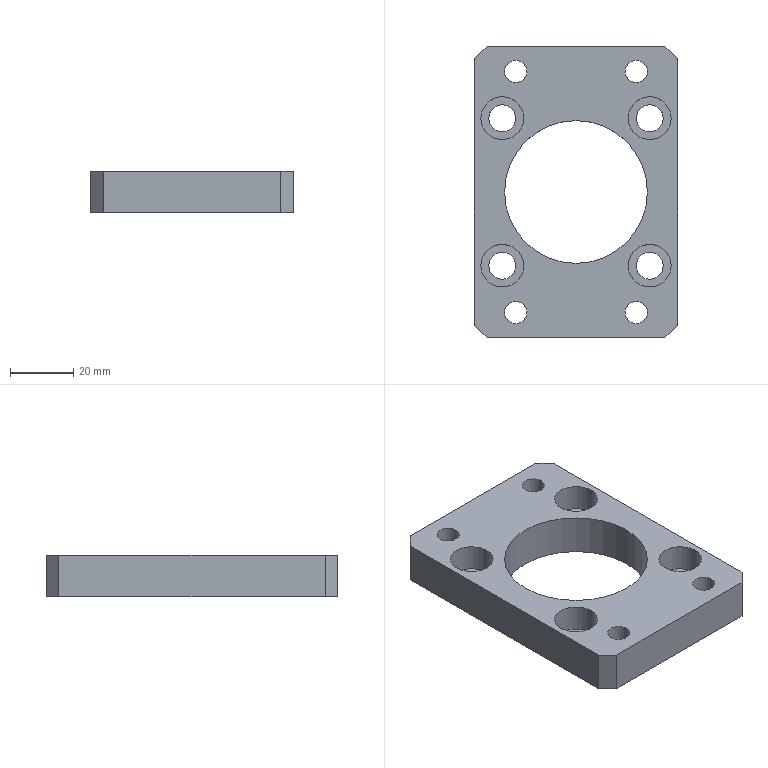Part | SolidWorks | features BaseBody 1 | 1 solid | 40 faces | box 64 x 92 x 13 mm | volume 47563 mm3 | cylinder 26 | plane 14 | commonest cylinder face diameters 7 x8 8.5 x8 13.5 x8 45 x2
STEP:
#1=CARTESIAN_POINT('',(22.5,0.,0.));
#2=VERTEX_POINT('',#1);
#3=CARTESIAN_POINT('',(-22.5,0.,0.));
#4=VERTEX_POINT('',#3);
#5=CARTESIAN_POINT('',(0.,0.,0.));
#6=DIRECTION('',(0.,0.,-1.));
#7=DIRECTION('',(1.,0.,0.));
#8=AXIS2_PLACEMENT_3D('',#5,#6,#7);
#9=CIRCLE('',#8,22.5);
#10=EDGE_CURVE('',#2,#4,#9,.T.);
#11=ORIENTED_EDGE('',*,*,#10,.T.);
#12=CARTESIAN_POINT('',(-22.5,0.,13.));
#13=VERTEX_POINT('',#12);
#14=CARTESIAN_POINT('',(-22.5,0.,0.));
#15=DIRECTION('',(0.,0.,1.));
#16=VECTOR('',#15,1000.);
#17=LINE('',#14,#16);
#18=EDGE_CURVE('',#4,#13,#17,.T.);
#19=ORIENTED_EDGE('',*,*,#18,.T.);
#20=CARTESIAN_POINT('',(22.5,0.,13.));
#21=VERTEX_POINT('',#20);
#22=CARTESIAN_POINT('',(0.,0.,13.));
#23=DIRECTION('',(0.,0.,-1.));
#24=DIRECTION('',(1.,0.,0.));
#25=AXIS2_PLACEMENT_3D('',#22,#23,#24);
#26=CIRCLE('',#25,22.5);
#27=EDGE_CURVE('',#21,#13,#26,.T.);
#28=ORIENTED_EDGE('',*,*,#27,.F.);
#29=CARTESIAN_POINT('',(22.5,0.,0.));
#30=DIRECTION('',(0.,0.,1.));
#31=VECTOR('',#30,1000.);
#32=LINE('',#29,#31);
#33=EDGE_CURVE('',#2,#21,#32,.T.);
#34=ORIENTED_EDGE('',*,*,#33,.F.);
#35=EDGE_LOOP('',(#11,#19,#28,#34));
#36=FACE_OUTER_BOUND('',#35,.T.);
#37=CARTESIAN_POINT('',(0.,0.,0.));
#38=DIRECTION('',(0.,0.,1.));
#39=DIRECTION('',(1.,0.,0.));
#40=AXIS2_PLACEMENT_3D('',#37,#38,#39);
#41=CYLINDRICAL_SURFACE('',#40,22.5);
#42=ADVANCED_FACE('',(#36),#41,.F.);
#43=CARTESIAN_POINT('',(-15.5,38.,0.));
#44=VERTEX_POINT('',#43);
#45=CARTESIAN_POINT('',(-22.5,38.,0.));
#46=VERTEX_POINT('',#45);
#47=CARTESIAN_POINT('',(-19.,38.,0.));
#48=DIRECTION('',(0.,0.,-1.));
#49=DIRECTION('',(1.,0.,0.));
#50=AXIS2_PLACEMENT_3D('',#47,#48,#49);
#51=CIRCLE('',#50,3.5);
#52=EDGE_CURVE('',#44,#46,#51,.T.);
#53=ORIENTED_EDGE('',*,*,#52,.T.);
#54=CARTESIAN_POINT('',(-22.5,38.,13.));
#55=VERTEX_POINT('',#54);
#56=CARTESIAN_POINT('',(-22.5,38.,0.));
#57=DIRECTION('',(0.,0.,1.));
#58=VECTOR('',#57,1000.);
#59=LINE('',#56,#58);
#60=EDGE_CURVE('',#46,#55,#59,.T.);
#61=ORIENTED_EDGE('',*,*,#60,.T.);
#62=CARTESIAN_POINT('',(-15.5,38.,13.));
#63=VERTEX_POINT('',#62);
#64=CARTESIAN_POINT('',(-19.,38.,13.));
#65=DIRECTION('',(0.,0.,-1.));
#66=DIRECTION('',(1.,0.,0.));
#67=AXIS2_PLACEMENT_3D('',#64,#65,#66);
#68=CIRCLE('',#67,3.5);
#69=EDGE_CURVE('',#63,#55,#68,.T.);
#70=ORIENTED_EDGE('',*,*,#69,.F.);
#71=CARTESIAN_POINT('',(-15.5,38.,0.));
#72=DIRECTION('',(0.,0.,1.));
#73=VECTOR('',#72,1000.);
#74=LINE('',#71,#73);
#75=EDGE_CURVE('',#44,#63,#74,.T.);
#76=ORIENTED_EDGE('',*,*,#75,.F.);
#77=EDGE_LOOP('',(#53,#61,#70,#76));
#78=FACE_OUTER_BOUND('',#77,.T.);
#79=CARTESIAN_POINT('',(-19.,38.,0.));
#80=DIRECTION('',(0.,0.,1.));
#81=DIRECTION('',(1.,0.,0.));
#82=AXIS2_PLACEMENT_3D('',#79,#80,#81);
#83=CYLINDRICAL_SURFACE('',#82,3.5);
#84=ADVANCED_FACE('',(#78),#83,.F.);
#85=CARTESIAN_POINT('',(-15.5,-38.,0.));
#86=VERTEX_POINT('',#85);
#87=CARTESIAN_POINT('',(-22.5,-38.,0.));
#88=VERTEX_POINT('',#87);
#89=CARTESIAN_POINT('',(-19.,-38.,0.));
#90=DIRECTION('',(0.,0.,-1.));
#91=DIRECTION('',(1.,0.,0.));
#92=AXIS2_PLACEMENT_3D('',#89,#90,#91);
#93=CIRCLE('',#92,3.5);
#94=EDGE_CURVE('',#86,#88,#93,.T.);
#95=ORIENTED_EDGE('',*,*,#94,.T.);
#96=CARTESIAN_POINT('',(-22.5,-38.,13.));
#97=VERTEX_POINT('',#96);
#98=CARTESIAN_POINT('',(-22.5,-38.,0.));
#99=DIRECTION('',(0.,0.,1.));
#100=VECTOR('',#99,1000.);
#101=LINE('',#98,#100);
#102=EDGE_CURVE('',#88,#97,#101,.T.);
#103=ORIENTED_EDGE('',*,*,#102,.T.);
#104=CARTESIAN_POINT('',(-15.5,-38.,13.));
#105=VERTEX_POINT('',#104);
#106=CARTESIAN_POINT('',(-19.,-38.,13.));
#107=DIRECTION('',(0.,0.,-1.));
#108=DIRECTION('',(1.,0.,0.));
#109=AXIS2_PLACEMENT_3D('',#106,#107,#108);
#110=CIRCLE('',#109,3.5);
#111=EDGE_CURVE('',#105,#97,#110,.T.);
#112=ORIENTED_EDGE('',*,*,#111,.F.);
#113=CARTESIAN_POINT('',(-15.5,-38.,0.));
#114=DIRECTION('',(0.,0.,1.));
#115=VECTOR('',#114,1000.);
#116=LINE('',#113,#115);
#117=EDGE_CURVE('',#86,#105,#116,.T.);
#118=ORIENTED_EDGE('',*,*,#117,.F.);
#119=EDGE_LOOP('',(#95,#103,#112,#118));
#120=FACE_OUTER_BOUND('',#119,.T.);
#121=CARTESIAN_POINT('',(-19.,-38.,0.));
#122=DIRECTION('',(0.,0.,1.));
#123=DIRECTION('',(1.,0.,0.));
#124=AXIS2_PLACEMENT_3D('',#121,#122,#123);
#125=CYLINDRICAL_SURFACE('',#124,3.5);
#126=ADVANCED_FACE('',(#120),#125,.F.);
#127=CARTESIAN_POINT('',(22.5,-38.,0.));
#128=VERTEX_POINT('',#127);
#129=CARTESIAN_POINT('',(15.5,-38.,0.));
#130=VERTEX_POINT('',#129);
#131=CARTESIAN_POINT('',(19.,-38.,0.));
#132=DIRECTION('',(0.,0.,-1.));
#133=DIRECTION('',(1.,0.,0.));
#134=AXIS2_PLACEMENT_3D('',#131,#132,#133);
#135=CIRCLE('',#134,3.5);
#136=EDGE_CURVE('',#128,#130,#135,.T.);
#137=ORIENTED_EDGE('',*,*,#136,.T.);
#138=CARTESIAN_POINT('',(15.5,-38.,13.));
#139=VERTEX_POINT('',#138);
#140=CARTESIAN_POINT('',(15.5,-38.,0.));
#141=DIRECTION('',(0.,0.,1.));
#142=VECTOR('',#141,1000.);
#143=LINE('',#140,#142);
#144=EDGE_CURVE('',#130,#139,#143,.T.);
#145=ORIENTED_EDGE('',*,*,#144,.T.);
#146=CARTESIAN_POINT('',(22.5,-38.,13.));
#147=VERTEX_POINT('',#146);
#148=CARTESIAN_POINT('',(19.,-38.,13.));
#149=DIRECTION('',(0.,0.,-1.));
#150=DIRECTION('',(1.,0.,0.));
#151=AXIS2_PLACEMENT_3D('',#148,#149,#150);
#152=CIRCLE('',#151,3.5);
#153=EDGE_CURVE('',#147,#139,#152,.T.);
#154=ORIENTED_EDGE('',*,*,#153,.F.);
#155=CARTESIAN_POINT('',(22.5,-38.,0.));
#156=DIRECTION('',(0.,0.,1.));
#157=VECTOR('',#156,1000.);
#158=LINE('',#155,#157);
#159=EDGE_CURVE('',#128,#147,#158,.T.);
#160=ORIENTED_EDGE('',*,*,#159,.F.);
#161=EDGE_LOOP('',(#137,#145,#154,#160));
#162=FACE_OUTER_BOUND('',#161,.T.);
#163=CARTESIAN_POINT('',(19.,-38.,0.));
#164=DIRECTION('',(0.,0.,1.));
#165=DIRECTION('',(1.,0.,0.));
#166=AXIS2_PLACEMENT_3D('',#163,#164,#165);
#167=CYLINDRICAL_SURFACE('',#166,3.5);
#168=ADVANCED_FACE('',(#162),#167,.F.);
#169=CARTESIAN_POINT('',(22.5,38.,0.));
#170=VERTEX_POINT('',#169);
#171=CARTESIAN_POINT('',(15.5,38.,0.));
#172=VERTEX_POINT('',#171);
#173=CARTESIAN_POINT('',(19.,38.,0.));
#174=DIRECTION('',(0.,0.,-1.));
#175=DIRECTION('',(1.,0.,0.));
#176=AXIS2_PLACEMENT_3D('',#173,#174,#175);
#177=CIRCLE('',#176,3.5);
#178=EDGE_CURVE('',#170,#172,#177,.T.);
#179=ORIENTED_EDGE('',*,*,#178,.T.);
#180=CARTESIAN_POINT('',(15.5,38.,13.));
#181=VERTEX_POINT('',#180);
#182=CARTESIAN_POINT('',(15.5,38.,0.));
#183=DIRECTION('',(0.,0.,1.));
#184=VECTOR('',#183,1000.);
#185=LINE('',#182,#184);
#186=EDGE_CURVE('',#172,#181,#185,.T.);
#187=ORIENTED_EDGE('',*,*,#186,.T.);
#188=CARTESIAN_POINT('',(22.5,38.,13.));
#189=VERTEX_POINT('',#188);
#190=CARTESIAN_POINT('',(19.,38.,13.));
#191=DIRECTION('',(0.,0.,-1.));
#192=DIRECTION('',(1.,0.,0.));
#193=AXIS2_PLACEMENT_3D('',#190,#191,#192);
#194=CIRCLE('',#193,3.5);
#195=EDGE_CURVE('',#189,#181,#194,.T.);
#196=ORIENTED_EDGE('',*,*,#195,.F.);
#197=CARTESIAN_POINT('',(22.5,38.,0.));
#198=DIRECTION('',(0.,0.,1.));
#199=VECTOR('',#198,1000.);
#200=LINE('',#197,#199);
#201=EDGE_CURVE('',#170,#189,#200,.T.);
#202=ORIENTED_EDGE('',*,*,#201,.F.);
#203=EDGE_LOOP('',(#179,#187,#196,#202));
#204=FACE_OUTER_BOUND('',#203,.T.);
#205=CARTESIAN_POINT('',(19.,38.,0.));
#206=DIRECTION('',(0.,0.,1.));
#207=DIRECTION('',(1.,0.,0.));
#208=AXIS2_PLACEMENT_3D('',#205,#206,#207);
#209=CYLINDRICAL_SURFACE('',#208,3.5);
#210=ADVANCED_FACE('',(#204),#209,.F.);
#211=CARTESIAN_POINT('',(-19.,-23.25,0.));
#212=VERTEX_POINT('',#211);
#213=CARTESIAN_POINT('',(-27.5,-23.25,0.));
#214=VERTEX_POINT('',#213);
#215=CARTESIAN_POINT('',(-23.25,-23.25,0.));
#216=DIRECTION('',(0.,0.,-1.));
#217=DIRECTION('',(1.,0.,0.));
#218=AXIS2_PLACEMENT_3D('',#215,#216,#217);
#219=CIRCLE('',#218,4.25);
#220=EDGE_CURVE('',#212,#214,#219,.T.);
#221=ORIENTED_EDGE('',*,*,#220,.T.);
#222=CARTESIAN_POINT('',(-27.5,-23.25,4.5));
#223=VERTEX_POINT('',#222);
#224=CARTESIAN_POINT('',(-27.5,-23.25,13.));
#225=DIRECTION('',(0.,0.,1.));
#226=VECTOR('',#225,1000.);
#227=LINE('',#224,#226);
#228=EDGE_CURVE('',#214,#223,#227,.T.);
#229=ORIENTED_EDGE('',*,*,#228,.T.);
#230=CARTESIAN_POINT('',(-19.,-23.25,4.5));
#231=VERTEX_POINT('',#230);
#232=CARTESIAN_POINT('',(-23.25,-23.25,4.5));
#233=DIRECTION('',(0.,0.,-1.));
#234=DIRECTION('',(1.,0.,0.));
#235=AXIS2_PLACEMENT_3D('',#232,#233,#234);
#236=CIRCLE('',#235,4.25);
#237=EDGE_CURVE('',#231,#223,#236,.T.);
#238=ORIENTED_EDGE('',*,*,#237,.F.);
#239=CARTESIAN_POINT('',(-19.,-23.25,13.));
#240=DIRECTION('',(0.,0.,1.));
#241=VECTOR('',#240,1000.);
#242=LINE('',#239,#241);
#243=EDGE_CURVE('',#212,#231,#242,.T.);
#244=ORIENTED_EDGE('',*,*,#243,.F.);
#245=EDGE_LOOP('',(#221,#229,#238,#244));
#246=FACE_OUTER_BOUND('',#245,.T.);
#247=CARTESIAN_POINT('',(-23.25,-23.25,13.));
#248=DIRECTION('',(0.,0.,1.));
#249=DIRECTION('',(1.,0.,0.));
#250=AXIS2_PLACEMENT_3D('',#247,#248,#249);
#251=CYLINDRICAL_SURFACE('',#250,4.25);
#252=ADVANCED_FACE('',(#246),#251,.F.);
#253=CARTESIAN_POINT('',(27.5,-23.25,0.));
#254=VERTEX_POINT('',#253);
#255=CARTESIAN_POINT('',(19.,-23.25,0.));
#256=VERTEX_POINT('',#255);
#257=CARTESIAN_POINT('',(23.25,-23.25,0.));
#258=DIRECTION('',(0.,0.,-1.));
#259=DIRECTION('',(1.,0.,0.));
#260=AXIS2_PLACEMENT_3D('',#257,#258,#259);
#261=CIRCLE('',#260,4.25);
#262=EDGE_CURVE('',#254,#256,#261,.T.);
#263=ORIENTED_EDGE('',*,*,#262,.T.);
#264=CARTESIAN_POINT('',(19.,-23.25,4.5));
#265=VERTEX_POINT('',#264);
#266=CARTESIAN_POINT('',(19.,-23.25,13.));
#267=DIRECTION('',(0.,0.,1.));
#268=VECTOR('',#267,1000.);
#269=LINE('',#266,#268);
#270=EDGE_CURVE('',#256,#265,#269,.T.);
#271=ORIENTED_EDGE('',*,*,#270,.T.);
#272=CARTESIAN_POINT('',(27.5,-23.25,4.5));
#273=VERTEX_POINT('',#272);
#274=CARTESIAN_POINT('',(23.25,-23.25,4.5));
#275=DIRECTION('',(0.,0.,-1.));
#276=DIRECTION('',(1.,0.,0.));
#277=AXIS2_PLACEMENT_3D('',#274,#275,#276);
#278=CIRCLE('',#277,4.25);
#279=EDGE_CURVE('',#273,#265,#278,.T.);
#280=ORIENTED_EDGE('',*,*,#279,.F.);
#281=CARTESIAN_POINT('',(27.5,-23.25,13.));
#282=DIRECTION('',(0.,0.,1.));
#283=VECTOR('',#282,1000.);
#284=LINE('',#281,#283);
#285=EDGE_CURVE('',#254,#273,#284,.T.);
#286=ORIENTED_EDGE('',*,*,#285,.F.);
#287=EDGE_LOOP('',(#263,#271,#280,#286));
#288=FACE_OUTER_BOUND('',#287,.T.);
#289=CARTESIAN_POINT('',(23.25,-23.25,13.));
#290=DIRECTION('',(0.,0.,1.));
#291=DIRECTION('',(1.,0.,0.));
#292=AXIS2_PLACEMENT_3D('',#289,#290,#291);
#293=CYLINDRICAL_SURFACE('',#292,4.25);
#294=ADVANCED_FACE('',(#288),#293,.F.);
#295=CARTESIAN_POINT('',(27.5,23.25,0.));
#296=VERTEX_POINT('',#295);
#297=CARTESIAN_POINT('',(19.,23.25,0.));
#298=VERTEX_POINT('',#297);
#299=CARTESIAN_POINT('',(23.25,23.25,0.));
#300=DIRECTION('',(0.,0.,-1.));
#301=DIRECTION('',(1.,0.,0.));
#302=AXIS2_PLACEMENT_3D('',#299,#300,#301);
#303=CIRCLE('',#302,4.25);
#304=EDGE_CURVE('',#296,#298,#303,.T.);
#305=ORIENTED_EDGE('',*,*,#304,.T.);
#306=CARTESIAN_POINT('',(19.,23.25,4.5));
#307=VERTEX_POINT('',#306);
#308=CARTESIAN_POINT('',(19.,23.25,13.));
#309=DIRECTION('',(0.,0.,1.));
#310=VECTOR('',#309,1000.);
#311=LINE('',#308,#310);
#312=EDGE_CURVE('',#298,#307,#311,.T.);
#313=ORIENTED_EDGE('',*,*,#312,.T.);
#314=CARTESIAN_POINT('',(27.5,23.25,4.5));
#315=VERTEX_POINT('',#314);
#316=CARTESIAN_POINT('',(23.25,23.25,4.5));
#317=DIRECTION('',(0.,0.,-1.));
#318=DIRECTION('',(1.,0.,0.));
#319=AXIS2_PLACEMENT_3D('',#316,#317,#318);
#320=CIRCLE('',#319,4.25);
#321=EDGE_CURVE('',#315,#307,#320,.T.);
#322=ORIENTED_EDGE('',*,*,#321,.F.);
#323=CARTESIAN_POINT('',(27.5,23.25,13.));
#324=DIRECTION('',(0.,0.,1.));
#325=VECTOR('',#324,1000.);
#326=LINE('',#323,#325);
#327=EDGE_CURVE('',#296,#315,#326,.T.);
#328=ORIENTED_EDGE('',*,*,#327,.F.);
#329=EDGE_LOOP('',(#305,#313,#322,#328));
#330=FACE_OUTER_BOUND('',#329,.T.);
#331=CARTESIAN_POINT('',(23.25,23.25,13.));
#332=DIRECTION('',(0.,0.,1.));
#333=DIRECTION('',(1.,0.,0.));
#334=AXIS2_PLACEMENT_3D('',#331,#332,#333);
#335=CYLINDRICAL_SURFACE('',#334,4.25);
#336=ADVANCED_FACE('',(#330),#335,.F.);
#337=CARTESIAN_POINT('',(-19.,23.25,0.));
#338=VERTEX_POINT('',#337);
#339=CARTESIAN_POINT('',(-27.5,23.25,0.));
#340=VERTEX_POINT('',#339);
#341=CARTESIAN_POINT('',(-23.25,23.25,0.));
#342=DIRECTION('',(0.,0.,-1.));
#343=DIRECTION('',(1.,0.,0.));
#344=AXIS2_PLACEMENT_3D('',#341,#342,#343);
#345=CIRCLE('',#344,4.25);
#346=EDGE_CURVE('',#338,#340,#345,.T.);
#347=ORIENTED_EDGE('',*,*,#346,.T.);
#348=CARTESIAN_POINT('',(-27.5,23.25,4.5));
#349=VERTEX_POINT('',#348);
#350=CARTESIAN_POINT('',(-27.5,23.25,13.));
#351=DIRECTION('',(0.,0.,1.));
#352=VECTOR('',#351,1000.);
#353=LINE('',#350,#352);
#354=EDGE_CURVE('',#340,#349,#353,.T.);
#355=ORIENTED_EDGE('',*,*,#354,.T.);
#356=CARTESIAN_POINT('',(-19.,23.25,4.5));
#357=VERTEX_POINT('',#356);
#358=CARTESIAN_POINT('',(-23.25,23.25,4.5));
#359=DIRECTION('',(0.,0.,-1.));
#360=DIRECTION('',(1.,0.,0.));
#361=AXIS2_PLACEMENT_3D('',#358,#359,#360);
#362=CIRCLE('',#361,4.25);
#363=EDGE_CURVE('',#357,#349,#362,.T.);
#364=ORIENTED_EDGE('',*,*,#363,.F.);
#365=CARTESIAN_POINT('',(-19.,23.25,13.));
#366=DIRECTION('',(0.,0.,1.));
#367=VECTOR('',#366,1000.);
#368=LINE('',#365,#367);
#369=EDGE_CURVE('',#338,#357,#368,.T.);
#370=ORIENTED_EDGE('',*,*,#369,.F.);
#371=EDGE_LOOP('',(#347,#355,#364,#370));
#372=FACE_OUTER_BOUND('',#371,.T.);
#373=CARTESIAN_POINT('',(-23.25,23.25,13.));
#374=DIRECTION('',(0.,0.,1.));
#375=DIRECTION('',(1.,0.,0.));
#376=AXIS2_PLACEMENT_3D('',#373,#374,#375);
#377=CYLINDRICAL_SURFACE('',#376,4.25);
#378=ADVANCED_FACE('',(#372),#377,.F.);
#379=CARTESIAN_POINT('',(-16.5,-23.25,4.5));
#380=VERTEX_POINT('',#379);
#381=CARTESIAN_POINT('',(-30.,-23.25,4.5));
#382=VERTEX_POINT('',#381);
#383=CARTESIAN_POINT('',(-23.25,-23.25,4.5));
#384=DIRECTION('',(0.,0.,-1.));
#385=DIRECTION('',(1.,0.,0.));
#386=AXIS2_PLACEMENT_3D('',#383,#384,#385);
#387=CIRCLE('',#386,6.75);
#388=EDGE_CURVE('',#380,#382,#387,.T.);
#389=ORIENTED_EDGE('',*,*,#388,.T.);
#390=CARTESIAN_POINT('',(-30.,-23.25,13.));
#391=VERTEX_POINT('',#390);
#392=CARTESIAN_POINT('',(-30.,-23.25,13.));
#393=DIRECTION('',(0.,0.,1.));
#394=VECTOR('',#393,1000.);
#395=LINE('',#392,#394);
#396=EDGE_CURVE('',#382,#391,#395,.T.);
#397=ORIENTED_EDGE('',*,*,#396,.T.);
#398=CARTESIAN_POINT('',(-16.5,-23.25,13.));
#399=VERTEX_POINT('',#398);
#400=CARTESIAN_POINT('',(-23.25,-23.25,13.));
#401=DIRECTION('',(0.,0.,-1.));
#402=DIRECTION('',(1.,0.,0.));
#403=AXIS2_PLACEMENT_3D('',#400,#401,#402);
#404=CIRCLE('',#403,6.75);
#405=EDGE_CURVE('',#399,#391,#404,.T.);
#406=ORIENTED_EDGE('',*,*,#405,.F.);
#407=CARTESIAN_POINT('',(-16.5,-23.25,13.));
#408=DIRECTION('',(0.,0.,1.));
#409=VECTOR('',#408,1000.);
#410=LINE('',#407,#409);
#411=EDGE_CURVE('',#380,#399,#410,.T.);
#412=ORIENTED_EDGE('',*,*,#411,.F.);
#413=EDGE_LOOP('',(#389,#397,#406,#412));
#414=FACE_OUTER_BOUND('',#413,.T.);
#415=CARTESIAN_POINT('',(-23.25,-23.25,13.));
#416=DIRECTION('',(0.,0.,1.));
#417=DIRECTION('',(1.,0.,0.));
#418=AXIS2_PLACEMENT_3D('',#415,#416,#417);
#419=CYLINDRICAL_SURFACE('',#418,6.75);
#420=ADVANCED_FACE('',(#414),#419,.F.);
#421=CARTESIAN_POINT('',(30.,-23.25,4.5));
#422=VERTEX_POINT('',#421);
#423=CARTESIAN_POINT('',(16.5,-23.25,4.5));
#424=VERTEX_POINT('',#423);
#425=CARTESIAN_POINT('',(23.25,-23.25,4.5));
#426=DIRECTION('',(0.,0.,-1.));
#427=DIRECTION('',(1.,0.,0.));
#428=AXIS2_PLACEMENT_3D('',#425,#426,#427);
#429=CIRCLE('',#428,6.75);
#430=EDGE_CURVE('',#422,#424,#429,.T.);
#431=ORIENTED_EDGE('',*,*,#430,.T.);
#432=CARTESIAN_POINT('',(16.5,-23.25,13.));
#433=VERTEX_POINT('',#432);
#434=CARTESIAN_POINT('',(16.5,-23.25,13.));
#435=DIRECTION('',(0.,0.,1.));
#436=VECTOR('',#435,1000.);
#437=LINE('',#434,#436);
#438=EDGE_CURVE('',#424,#433,#437,.T.);
#439=ORIENTED_EDGE('',*,*,#438,.T.);
#440=CARTESIAN_POINT('',(30.,-23.25,13.));
#441=VERTEX_POINT('',#440);
#442=CARTESIAN_POINT('',(23.25,-23.25,13.));
#443=DIRECTION('',(0.,0.,-1.));
#444=DIRECTION('',(1.,0.,0.));
#445=AXIS2_PLACEMENT_3D('',#442,#443,#444);
#446=CIRCLE('',#445,6.75);
#447=EDGE_CURVE('',#441,#433,#446,.T.);
#448=ORIENTED_EDGE('',*,*,#447,.F.);
#449=CARTESIAN_POINT('',(30.,-23.25,13.));
#450=DIRECTION('',(0.,0.,1.));
#451=VECTOR('',#450,1000.);
#452=LINE('',#449,#451);
#453=EDGE_CURVE('',#422,#441,#452,.T.);
#454=ORIENTED_EDGE('',*,*,#453,.F.);
#455=EDGE_LOOP('',(#431,#439,#448,#454));
#456=FACE_OUTER_BOUND('',#455,.T.);
#457=CARTESIAN_POINT('',(23.25,-23.25,13.));
#458=DIRECTION('',(0.,0.,1.));
#459=DIRECTION('',(1.,0.,0.));
#460=AXIS2_PLACEMENT_3D('',#457,#458,#459);
#461=CYLINDRICAL_SURFACE('',#460,6.75);
#462=ADVANCED_FACE('',(#456),#461,.F.);
#463=CARTESIAN_POINT('',(30.,23.25,4.5));
#464=VERTEX_POINT('',#463);
#465=CARTESIAN_POINT('',(16.5,23.25,4.5));
#466=VERTEX_POINT('',#465);
#467=CARTESIAN_POINT('',(23.25,23.25,4.5));
#468=DIRECTION('',(0.,0.,-1.));
#469=DIRECTION('',(1.,0.,0.));
#470=AXIS2_PLACEMENT_3D('',#467,#468,#469);
#471=CIRCLE('',#470,6.75);
#472=EDGE_CURVE('',#464,#466,#471,.T.);
#473=ORIENTED_EDGE('',*,*,#472,.T.);
#474=CARTESIAN_POINT('',(16.5,23.25,13.));
#475=VERTEX_POINT('',#474);
#476=CARTESIAN_POINT('',(16.5,23.25,13.));
#477=DIRECTION('',(0.,0.,1.));
#478=VECTOR('',#477,1000.);
#479=LINE('',#476,#478);
#480=EDGE_CURVE('',#466,#475,#479,.T.);
#481=ORIENTED_EDGE('',*,*,#480,.T.);
#482=CARTESIAN_POINT('',(30.,23.25,13.));
#483=VERTEX_POINT('',#482);
#484=CARTESIAN_POINT('',(23.25,23.25,13.));
#485=DIRECTION('',(0.,0.,-1.));
#486=DIRECTION('',(1.,0.,0.));
#487=AXIS2_PLACEMENT_3D('',#484,#485,#486);
#488=CIRCLE('',#487,6.75);
#489=EDGE_CURVE('',#483,#475,#488,.T.);
#490=ORIENTED_EDGE('',*,*,#489,.F.);
#491=CARTESIAN_POINT('',(30.,23.25,13.));
#492=DIRECTION('',(0.,0.,1.));
#493=VECTOR('',#492,1000.);
#494=LINE('',#491,#493);
#495=EDGE_CURVE('',#464,#483,#494,.T.);
#496=ORIENTED_EDGE('',*,*,#495,.F.);
#497=EDGE_LOOP('',(#473,#481,#490,#496));
#498=FACE_OUTER_BOUND('',#497,.T.);
#499=CARTESIAN_POINT('',(23.25,23.25,13.));
#500=DIRECTION('',(0.,0.,1.));
#501=DIRECTION('',(1.,0.,0.));
#502=AXIS2_PLACEMENT_3D('',#499,#500,#501);
#503=CYLINDRICAL_SURFACE('',#502,6.75);
#504=ADVANCED_FACE('',(#498),#503,.F.);
#505=CARTESIAN_POINT('',(-16.5,23.25,4.5));
#506=VERTEX_POINT('',#505);
#507=CARTESIAN_POINT('',(-30.,23.25,4.5));
#508=VERTEX_POINT('',#507);
#509=CARTESIAN_POINT('',(-23.25,23.25,4.5));
#510=DIRECTION('',(0.,0.,-1.));
#511=DIRECTION('',(1.,0.,0.));
#512=AXIS2_PLACEMENT_3D('',#509,#510,#511);
#513=CIRCLE('',#512,6.75);
#514=EDGE_CURVE('',#506,#508,#513,.T.);
#515=ORIENTED_EDGE('',*,*,#514,.T.);
#516=CARTESIAN_POINT('',(-30.,23.25,13.));
#517=VERTEX_POINT('',#516);
#518=CARTESIAN_POINT('',(-30.,23.25,13.));
#519=DIRECTION('',(0.,0.,1.));
#520=VECTOR('',#519,1000.);
#521=LINE('',#518,#520);
#522=EDGE_CURVE('',#508,#517,#521,.T.);
#523=ORIENTED_EDGE('',*,*,#522,.T.);
#524=CARTESIAN_POINT('',(-16.5,23.25,13.));
#525=VERTEX_POINT('',#524);
#526=CARTESIAN_POINT('',(-23.25,23.25,13.));
#527=DIRECTION('',(0.,0.,-1.));
#528=DIRECTION('',(1.,0.,0.));
#529=AXIS2_PLACEMENT_3D('',#526,#527,#528);
#530=CIRCLE('',#529,6.75);
#531=EDGE_CURVE('',#525,#517,#530,.T.);
#532=ORIENTED_EDGE('',*,*,#531,.F.);
#533=CARTESIAN_POINT('',(-16.5,23.25,13.));
#534=DIRECTION('',(0.,0.,1.));
#535=VECTOR('',#534,1000.);
#536=LINE('',#533,#535);
#537=EDGE_CURVE('',#506,#525,#536,.T.);
#538=ORIENTED_EDGE('',*,*,#537,.F.);
#539=EDGE_LOOP('',(#515,#523,#532,#538));
#540=FACE_OUTER_BOUND('',#539,.T.);
#541=CARTESIAN_POINT('',(-23.25,23.25,13.));
#542=DIRECTION('',(0.,0.,1.));
#543=DIRECTION('',(1.,0.,0.));
#544=AXIS2_PLACEMENT_3D('',#541,#542,#543);
#545=CYLINDRICAL_SURFACE('',#544,6.75);
#546=ADVANCED_FACE('',(#540),#545,.F.);
#547=CARTESIAN_POINT('',(-32.,-42.,0.));
#548=VERTEX_POINT('',#547);
#549=CARTESIAN_POINT('',(-28.,-46.,0.));
#550=VERTEX_POINT('',#549);
#551=CARTESIAN_POINT('',(-32.,-42.,0.));
#552=DIRECTION('',(0.7071,-0.7071,0.));
#553=VECTOR('',#552,1000.);
#554=LINE('',#551,#553);
#555=EDGE_CURVE('',#548,#550,#554,.T.);
#556=ORIENTED_EDGE('',*,*,#555,.F.);
#557=CARTESIAN_POINT('',(-32.,42.,0.));
#558=VERTEX_POINT('',#557);
#559=CARTESIAN_POINT('',(-32.,0.,0.));
#560=DIRECTION('',(0.,-1.,0.));
#561=VECTOR('',#560,1000.);
#562=LINE('',#559,#561);
#563=EDGE_CURVE('',#558,#548,#562,.T.);
#564=ORIENTED_EDGE('',*,*,#563,.F.);
#565=CARTESIAN_POINT('',(-28.,46.,0.));
#566=VERTEX_POINT('',#565);
#567=CARTESIAN_POINT('',(-28.,46.,0.));
#568=DIRECTION('',(-0.7071,-0.7071,0.));
#569=VECTOR('',#568,1000.);
#570=LINE('',#567,#569);
#571=EDGE_CURVE('',#566,#558,#570,.T.);
#572=ORIENTED_EDGE('',*,*,#571,.F.);
#573=CARTESIAN_POINT('',(28.,46.,0.));
#574=VERTEX_POINT('',#573);
#575=CARTESIAN_POINT('',(0.,46.,0.));
#576=DIRECTION('',(-1.,0.,0.));
#577=VECTOR('',#576,1000.);
#578=LINE('',#575,#577);
#579=EDGE_CURVE('',#574,#566,#578,.T.);
#580=ORIENTED_EDGE('',*,*,#579,.F.);
#581=CARTESIAN_POINT('',(32.,42.,0.));
#582=VERTEX_POINT('',#581);
#583=CARTESIAN_POINT('',(32.,42.,0.));
#584=DIRECTION('',(-0.7071,0.7071,0.));
#585=VECTOR('',#584,1000.);
#586=LINE('',#583,#585);
#587=EDGE_CURVE('',#582,#574,#586,.T.);
#588=ORIENTED_EDGE('',*,*,#587,.F.);
#589=CARTESIAN_POINT('',(32.,-42.,0.));
#590=VERTEX_POINT('',#589);
#591=CARTESIAN_POINT('',(32.,0.,0.));
#592=DIRECTION('',(0.,1.,0.));
#593=VECTOR('',#592,1000.);
#594=LINE('',#591,#593);
#595=EDGE_CURVE('',#590,#582,#594,.T.);
#596=ORIENTED_EDGE('',*,*,#595,.F.);
#597=CARTESIAN_POINT('',(28.,-46.,0.));
#598=VERTEX_POINT('',#597);
#599=CARTESIAN_POINT('',(28.,-46.,0.));
#600=DIRECTION('',(0.7071,0.7071,0.));
#601=VECTOR('',#600,1000.);
#602=LINE('',#599,#601);
#603=EDGE_CURVE('',#598,#590,#602,.T.);
#604=ORIENTED_EDGE('',*,*,#603,.F.);
#605=CARTESIAN_POINT('',(0.,-46.,0.));
#606=DIRECTION('',(1.,0.,0.));
#607=VECTOR('',#606,1000.);
#608=LINE('',#605,#607);
#609=EDGE_CURVE('',#550,#598,#608,.T.);
#610=ORIENTED_EDGE('',*,*,#609,.F.);
#611=EDGE_LOOP('',(#556,#564,#572,#580,#588,#596,#604,#610));
#612=FACE_OUTER_BOUND('',#611,.T.);
#613=ORIENTED_EDGE('',*,*,#10,.F.);
#614=CARTESIAN_POINT('',(0.,0.,0.));
#615=DIRECTION('',(0.,0.,-1.));
#616=DIRECTION('',(1.,0.,0.));
#617=AXIS2_PLACEMENT_3D('',#614,#615,#616);
#618=CIRCLE('',#617,22.5);
#619=EDGE_CURVE('',#4,#2,#618,.T.);
#620=ORIENTED_EDGE('',*,*,#619,.F.);
#621=EDGE_LOOP('',(#613,#620));
#622=FACE_BOUND('',#621,.T.);
#623=ORIENTED_EDGE('',*,*,#52,.F.);
#624=CARTESIAN_POINT('',(-19.,38.,0.));
#625=DIRECTION('',(0.,0.,-1.));
#626=DIRECTION('',(1.,0.,0.));
#627=AXIS2_PLACEMENT_3D('',#624,#625,#626);
#628=CIRCLE('',#627,3.5);
#629=EDGE_CURVE('',#46,#44,#628,.T.);
#630=ORIENTED_EDGE('',*,*,#629,.F.);
#631=EDGE_LOOP('',(#623,#630));
#632=FACE_BOUND('',#631,.T.);
#633=ORIENTED_EDGE('',*,*,#94,.F.);
#634=CARTESIAN_POINT('',(-19.,-38.,0.));
#635=DIRECTION('',(0.,0.,-1.));
#636=DIRECTION('',(1.,0.,0.));
#637=AXIS2_PLACEMENT_3D('',#634,#635,#636);
#638=CIRCLE('',#637,3.5);
#639=EDGE_CURVE('',#88,#86,#638,.T.);
#640=ORIENTED_EDGE('',*,*,#639,.F.);
#641=EDGE_LOOP('',(#633,#640));
#642=FACE_BOUND('',#641,.T.);
#643=ORIENTED_EDGE('',*,*,#136,.F.);
#644=CARTESIAN_POINT('',(19.,-38.,0.));
#645=DIRECTION('',(0.,0.,-1.));
#646=DIRECTION('',(1.,0.,0.));
#647=AXIS2_PLACEMENT_3D('',#644,#645,#646);
#648=CIRCLE('',#647,3.5);
#649=EDGE_CURVE('',#130,#128,#648,.T.);
#650=ORIENTED_EDGE('',*,*,#649,.F.);
#651=EDGE_LOOP('',(#643,#650));
#652=FACE_BOUND('',#651,.T.);
#653=ORIENTED_EDGE('',*,*,#178,.F.);
#654=CARTESIAN_POINT('',(19.,38.,0.));
#655=DIRECTION('',(0.,0.,-1.));
#656=DIRECTION('',(1.,0.,0.));
#657=AXIS2_PLACEMENT_3D('',#654,#655,#656);
#658=CIRCLE('',#657,3.5);
#659=EDGE_CURVE('',#172,#170,#658,.T.);
#660=ORIENTED_EDGE('',*,*,#659,.F.);
#661=EDGE_LOOP('',(#653,#660));
#662=FACE_BOUND('',#661,.T.);
#663=ORIENTED_EDGE('',*,*,#220,.F.);
#664=CARTESIAN_POINT('',(-23.25,-23.25,0.));
#665=DIRECTION('',(0.,0.,-1.));
#666=DIRECTION('',(1.,0.,0.));
#667=AXIS2_PLACEMENT_3D('',#664,#665,#666);
#668=CIRCLE('',#667,4.25);
#669=EDGE_CURVE('',#214,#212,#668,.T.);
#670=ORIENTED_EDGE('',*,*,#669,.F.);
#671=EDGE_LOOP('',(#663,#670));
#672=FACE_BOUND('',#671,.T.);
#673=ORIENTED_EDGE('',*,*,#262,.F.);
#674=CARTESIAN_POINT('',(23.25,-23.25,0.));
#675=DIRECTION('',(0.,0.,-1.));
#676=DIRECTION('',(1.,0.,0.));
#677=AXIS2_PLACEMENT_3D('',#674,#675,#676);
#678=CIRCLE('',#677,4.25);
#679=EDGE_CURVE('',#256,#254,#678,.T.);
#680=ORIENTED_EDGE('',*,*,#679,.F.);
#681=EDGE_LOOP('',(#673,#680));
#682=FACE_BOUND('',#681,.T.);
#683=ORIENTED_EDGE('',*,*,#304,.F.);
#684=CARTESIAN_POINT('',(23.25,23.25,0.));
#685=DIRECTION('',(0.,0.,-1.));
#686=DIRECTION('',(1.,0.,0.));
#687=AXIS2_PLACEMENT_3D('',#684,#685,#686);
#688=CIRCLE('',#687,4.25);
#689=EDGE_CURVE('',#298,#296,#688,.T.);
#690=ORIENTED_EDGE('',*,*,#689,.F.);
#691=EDGE_LOOP('',(#683,#690));
#692=FACE_BOUND('',#691,.T.);
#693=ORIENTED_EDGE('',*,*,#346,.F.);
#694=CARTESIAN_POINT('',(-23.25,23.25,0.));
#695=DIRECTION('',(0.,0.,-1.));
#696=DIRECTION('',(1.,0.,0.));
#697=AXIS2_PLACEMENT_3D('',#694,#695,#696);
#698=CIRCLE('',#697,4.25);
#699=EDGE_CURVE('',#340,#338,#698,.T.);
#700=ORIENTED_EDGE('',*,*,#699,.F.);
#701=EDGE_LOOP('',(#693,#700));
#702=FACE_BOUND('',#701,.T.);
#703=CARTESIAN_POINT('',(0.,0.,0.));
#704=DIRECTION('',(0.,0.,1.));
#705=DIRECTION('',(1.,0.,0.));
#706=AXIS2_PLACEMENT_3D('',#703,#704,#705);
#707=PLANE('',#706);
#708=ADVANCED_FACE('',(#612,#622,#632,#642,#652,#662,#672,#682,#692,#702),#707,.F.);
#709=CARTESIAN_POINT('',(-28.,-46.,13.));
#710=VERTEX_POINT('',#709);
#711=CARTESIAN_POINT('',(-28.,-46.,13.));
#712=DIRECTION('',(0.,0.,1.));
#713=VECTOR('',#712,1000.);
#714=LINE('',#711,#713);
#715=EDGE_CURVE('',#550,#710,#714,.T.);
#716=ORIENTED_EDGE('',*,*,#715,.F.);
#717=ORIENTED_EDGE('',*,*,#609,.T.);
#718=CARTESIAN_POINT('',(28.,-46.,13.));
#719=VERTEX_POINT('',#718);
#720=CARTESIAN_POINT('',(28.,-46.,13.));
#721=DIRECTION('',(0.,0.,-1.));
#722=VECTOR('',#721,1000.);
#723=LINE('',#720,#722);
#724=EDGE_CURVE('',#719,#598,#723,.T.);
#725=ORIENTED_EDGE('',*,*,#724,.F.);
#726=CARTESIAN_POINT('',(32.,-46.,13.));
#727=DIRECTION('',(1.,0.,0.));
#728=VECTOR('',#727,1000.);
#729=LINE('',#726,#728);
#730=EDGE_CURVE('',#710,#719,#729,.T.);
#731=ORIENTED_EDGE('',*,*,#730,.F.);
#732=EDGE_LOOP('',(#716,#717,#725,#731));
#733=FACE_OUTER_BOUND('',#732,.T.);
#734=CARTESIAN_POINT('',(32.,-46.,13.));
#735=DIRECTION('',(0.,1.,0.));
#736=DIRECTION('',(0.,0.,1.));
#737=AXIS2_PLACEMENT_3D('',#734,#735,#736);
#738=PLANE('',#737);
#739=ADVANCED_FACE('',(#733),#738,.F.);
#740=CARTESIAN_POINT('',(-32.,-42.,13.));
#741=VERTEX_POINT('',#740);
#742=CARTESIAN_POINT('',(-32.,-42.,13.));
#743=DIRECTION('',(0.,0.,1.));
#744=VECTOR('',#743,1000.);
#745=LINE('',#742,#744);
#746=EDGE_CURVE('',#548,#741,#745,.T.);
#747=ORIENTED_EDGE('',*,*,#746,.F.);
#748=ORIENTED_EDGE('',*,*,#555,.T.);
#749=ORIENTED_EDGE('',*,*,#715,.T.);
#750=CARTESIAN_POINT('',(-28.,-46.,13.));
#751=DIRECTION('',(0.7071,-0.7071,0.));
#752=VECTOR('',#751,1000.);
#753=LINE('',#750,#752);
#754=EDGE_CURVE('',#741,#710,#753,.T.);
#755=ORIENTED_EDGE('',*,*,#754,.F.);
#756=EDGE_LOOP('',(#747,#748,#749,#755));
#757=FACE_OUTER_BOUND('',#756,.T.);
#758=CARTESIAN_POINT('',(-28.,-46.,13.));
#759=DIRECTION('',(0.7071,0.7071,0.));
#760=DIRECTION('',(-0.7071,0.7071,0.));
#761=AXIS2_PLACEMENT_3D('',#758,#759,#760);
#762=PLANE('',#761);
#763=ADVANCED_FACE('',(#757),#762,.F.);
#764=ORIENTED_EDGE('',*,*,#746,.T.);
#765=CARTESIAN_POINT('',(-32.,42.,13.));
#766=VERTEX_POINT('',#765);
#767=CARTESIAN_POINT('',(-32.,-46.,13.));
#768=DIRECTION('',(0.,-1.,0.));
#769=VECTOR('',#768,1000.);
#770=LINE('',#767,#769);
#771=EDGE_CURVE('',#766,#741,#770,.T.);
#772=ORIENTED_EDGE('',*,*,#771,.F.);
#773=CARTESIAN_POINT('',(-32.,42.,13.));
#774=DIRECTION('',(0.,0.,1.));
#775=VECTOR('',#774,1000.);
#776=LINE('',#773,#775);
#777=EDGE_CURVE('',#558,#766,#776,.T.);
#778=ORIENTED_EDGE('',*,*,#777,.F.);
#779=ORIENTED_EDGE('',*,*,#563,.T.);
#780=EDGE_LOOP('',(#764,#772,#778,#779));
#781=FACE_OUTER_BOUND('',#780,.T.);
#782=CARTESIAN_POINT('',(-32.,-46.,13.));
#783=DIRECTION('',(1.,0.,0.));
#784=DIRECTION('',(0.,0.,-1.));
#785=AXIS2_PLACEMENT_3D('',#782,#783,#784);
#786=PLANE('',#785);
#787=ADVANCED_FACE('',(#781),#786,.F.);
#788=CARTESIAN_POINT('',(-28.,46.,13.));
#789=VERTEX_POINT('',#788);
#790=CARTESIAN_POINT('',(-28.,46.,13.));
#791=DIRECTION('',(0.,0.,1.));
#792=VECTOR('',#791,1000.);
#793=LINE('',#790,#792);
#794=EDGE_CURVE('',#566,#789,#793,.T.);
#795=ORIENTED_EDGE('',*,*,#794,.F.);
#796=ORIENTED_EDGE('',*,*,#571,.T.);
#797=ORIENTED_EDGE('',*,*,#777,.T.);
#798=CARTESIAN_POINT('',(-32.,42.,13.));
#799=DIRECTION('',(-0.7071,-0.7071,0.));
#800=VECTOR('',#799,1000.);
#801=LINE('',#798,#800);
#802=EDGE_CURVE('',#789,#766,#801,.T.);
#803=ORIENTED_EDGE('',*,*,#802,.F.);
#804=EDGE_LOOP('',(#795,#796,#797,#803));
#805=FACE_OUTER_BOUND('',#804,.T.);
#806=CARTESIAN_POINT('',(-32.,42.,13.));
#807=DIRECTION('',(0.7071,-0.7071,0.));
#808=DIRECTION('',(0.7071,0.7071,0.));
#809=AXIS2_PLACEMENT_3D('',#806,#807,#808);
#810=PLANE('',#809);
#811=ADVANCED_FACE('',(#805),#810,.F.);
#812=ORIENTED_EDGE('',*,*,#794,.T.);
#813=CARTESIAN_POINT('',(28.,46.,13.));
#814=VERTEX_POINT('',#813);
#815=CARTESIAN_POINT('',(32.,46.,13.));
#816=DIRECTION('',(-1.,0.,0.));
#817=VECTOR('',#816,1000.);
#818=LINE('',#815,#817);
#819=EDGE_CURVE('',#814,#789,#818,.T.);
#820=ORIENTED_EDGE('',*,*,#819,.F.);
#821=CARTESIAN_POINT('',(28.,46.,13.));
#822=DIRECTION('',(0.,0.,1.));
#823=VECTOR('',#822,1000.);
#824=LINE('',#821,#823);
#825=EDGE_CURVE('',#574,#814,#824,.T.);
#826=ORIENTED_EDGE('',*,*,#825,.F.);
#827=ORIENTED_EDGE('',*,*,#579,.T.);
#828=EDGE_LOOP('',(#812,#820,#826,#827));
#829=FACE_OUTER_BOUND('',#828,.T.);
#830=CARTESIAN_POINT('',(32.,46.,13.));
#831=DIRECTION('',(0.,-1.,0.));
#832=DIRECTION('',(0.,0.,-1.));
#833=AXIS2_PLACEMENT_3D('',#830,#831,#832);
#834=PLANE('',#833);
#835=ADVANCED_FACE('',(#829),#834,.F.);
#836=CARTESIAN_POINT('',(32.,42.,13.));
#837=VERTEX_POINT('',#836);
#838=CARTESIAN_POINT('',(32.,42.,13.));
#839=DIRECTION('',(0.,0.,1.));
#840=VECTOR('',#839,1000.);
#841=LINE('',#838,#840);
#842=EDGE_CURVE('',#582,#837,#841,.T.);
#843=ORIENTED_EDGE('',*,*,#842,.F.);
#844=ORIENTED_EDGE('',*,*,#587,.T.);
#845=ORIENTED_EDGE('',*,*,#825,.T.);
#846=CARTESIAN_POINT('',(28.,46.,13.));
#847=DIRECTION('',(-0.7071,0.7071,0.));
#848=VECTOR('',#847,1000.);
#849=LINE('',#846,#848);
#850=EDGE_CURVE('',#837,#814,#849,.T.);
#851=ORIENTED_EDGE('',*,*,#850,.F.);
#852=EDGE_LOOP('',(#843,#844,#845,#851));
#853=FACE_OUTER_BOUND('',#852,.T.);
#854=CARTESIAN_POINT('',(28.,46.,13.));
#855=DIRECTION('',(-0.7071,-0.7071,0.));
#856=DIRECTION('',(0.7071,-0.7071,0.));
#857=AXIS2_PLACEMENT_3D('',#854,#855,#856);
#858=PLANE('',#857);
#859=ADVANCED_FACE('',(#853),#858,.F.);
#860=CARTESIAN_POINT('',(32.,-42.,13.));
#861=VERTEX_POINT('',#860);
#862=CARTESIAN_POINT('',(32.,-42.,13.));
#863=DIRECTION('',(0.,0.,1.));
#864=VECTOR('',#863,1000.);
#865=LINE('',#862,#864);
#866=EDGE_CURVE('',#590,#861,#865,.T.);
#867=ORIENTED_EDGE('',*,*,#866,.F.);
#868=ORIENTED_EDGE('',*,*,#595,.T.);
#869=ORIENTED_EDGE('',*,*,#842,.T.);
#870=CARTESIAN_POINT('',(32.,-46.,13.));
#871=DIRECTION('',(0.,1.,0.));
#872=VECTOR('',#871,1000.);
#873=LINE('',#870,#872);
#874=EDGE_CURVE('',#861,#837,#873,.T.);
#875=ORIENTED_EDGE('',*,*,#874,.F.);
#876=EDGE_LOOP('',(#867,#868,#869,#875));
#877=FACE_OUTER_BOUND('',#876,.T.);
#878=CARTESIAN_POINT('',(32.,-46.,13.));
#879=DIRECTION('',(-1.,0.,0.));
#880=DIRECTION('',(0.,0.,1.));
#881=AXIS2_PLACEMENT_3D('',#878,#879,#880);
#882=PLANE('',#881);
#883=ADVANCED_FACE('',(#877),#882,.F.);
#884=ORIENTED_EDGE('',*,*,#724,.T.);
#885=ORIENTED_EDGE('',*,*,#603,.T.);
#886=ORIENTED_EDGE('',*,*,#866,.T.);
#887=CARTESIAN_POINT('',(32.,-42.,13.));
#888=DIRECTION('',(0.7071,0.7071,0.));
#889=VECTOR('',#888,1000.);
#890=LINE('',#887,#889);
#891=EDGE_CURVE('',#719,#861,#890,.T.);
#892=ORIENTED_EDGE('',*,*,#891,.F.);
#893=EDGE_LOOP('',(#884,#885,#886,#892));
#894=FACE_OUTER_BOUND('',#893,.T.);
#895=CARTESIAN_POINT('',(32.,-42.,13.));
#896=DIRECTION('',(-0.7071,0.7071,0.));
#897=DIRECTION('',(-0.7071,-0.7071,0.));
#898=AXIS2_PLACEMENT_3D('',#895,#896,#897);
#899=PLANE('',#898);
#900=ADVANCED_FACE('',(#894),#899,.F.);
#901=ORIENTED_EDGE('',*,*,#18,.F.);
#902=ORIENTED_EDGE('',*,*,#619,.T.);
#903=ORIENTED_EDGE('',*,*,#33,.T.);
#904=CARTESIAN_POINT('',(0.,0.,13.));
#905=DIRECTION('',(0.,0.,-1.));
#906=DIRECTION('',(1.,0.,0.));
#907=AXIS2_PLACEMENT_3D('',#904,#905,#906);
#908=CIRCLE('',#907,22.5);
#909=EDGE_CURVE('',#13,#21,#908,.T.);
#910=ORIENTED_EDGE('',*,*,#909,.F.);
#911=EDGE_LOOP('',(#901,#902,#903,#910));
#912=FACE_OUTER_BOUND('',#911,.T.);
#913=CARTESIAN_POINT('',(0.,0.,0.));
#914=DIRECTION('',(0.,0.,1.));
#915=DIRECTION('',(1.,0.,0.));
#916=AXIS2_PLACEMENT_3D('',#913,#914,#915);
#917=CYLINDRICAL_SURFACE('',#916,22.5);
#918=ADVANCED_FACE('',(#912),#917,.F.);
#919=ORIENTED_EDGE('',*,*,#60,.F.);
#920=ORIENTED_EDGE('',*,*,#629,.T.);
#921=ORIENTED_EDGE('',*,*,#75,.T.);
#922=CARTESIAN_POINT('',(-19.,38.,13.));
#923=DIRECTION('',(0.,0.,-1.));
#924=DIRECTION('',(1.,0.,0.));
#925=AXIS2_PLACEMENT_3D('',#922,#923,#924);
#926=CIRCLE('',#925,3.5);
#927=EDGE_CURVE('',#55,#63,#926,.T.);
#928=ORIENTED_EDGE('',*,*,#927,.F.);
#929=EDGE_LOOP('',(#919,#920,#921,#928));
#930=FACE_OUTER_BOUND('',#929,.T.);
#931=CARTESIAN_POINT('',(-19.,38.,0.));
#932=DIRECTION('',(0.,0.,1.));
#933=DIRECTION('',(1.,0.,0.));
#934=AXIS2_PLACEMENT_3D('',#931,#932,#933);
#935=CYLINDRICAL_SURFACE('',#934,3.5);
#936=ADVANCED_FACE('',(#930),#935,.F.);
#937=ORIENTED_EDGE('',*,*,#102,.F.);
#938=ORIENTED_EDGE('',*,*,#639,.T.);
#939=ORIENTED_EDGE('',*,*,#117,.T.);
#940=CARTESIAN_POINT('',(-19.,-38.,13.));
#941=DIRECTION('',(0.,0.,-1.));
#942=DIRECTION('',(1.,0.,0.));
#943=AXIS2_PLACEMENT_3D('',#940,#941,#942);
#944=CIRCLE('',#943,3.5);
#945=EDGE_CURVE('',#97,#105,#944,.T.);
#946=ORIENTED_EDGE('',*,*,#945,.F.);
#947=EDGE_LOOP('',(#937,#938,#939,#946));
#948=FACE_OUTER_BOUND('',#947,.T.);
#949=CARTESIAN_POINT('',(-19.,-38.,0.));
#950=DIRECTION('',(0.,0.,1.));
#951=DIRECTION('',(1.,0.,0.));
#952=AXIS2_PLACEMENT_3D('',#949,#950,#951);
#953=CYLINDRICAL_SURFACE('',#952,3.5);
#954=ADVANCED_FACE('',(#948),#953,.F.);
#955=ORIENTED_EDGE('',*,*,#144,.F.);
#956=ORIENTED_EDGE('',*,*,#649,.T.);
#957=ORIENTED_EDGE('',*,*,#159,.T.);
#958=CARTESIAN_POINT('',(19.,-38.,13.));
#959=DIRECTION('',(0.,0.,-1.));
#960=DIRECTION('',(1.,0.,0.));
#961=AXIS2_PLACEMENT_3D('',#958,#959,#960);
#962=CIRCLE('',#961,3.5);
#963=EDGE_CURVE('',#139,#147,#962,.T.);
#964=ORIENTED_EDGE('',*,*,#963,.F.);
#965=EDGE_LOOP('',(#955,#956,#957,#964));
#966=FACE_OUTER_BOUND('',#965,.T.);
#967=CARTESIAN_POINT('',(19.,-38.,0.));
#968=DIRECTION('',(0.,0.,1.));
#969=DIRECTION('',(1.,0.,0.));
#970=AXIS2_PLACEMENT_3D('',#967,#968,#969);
#971=CYLINDRICAL_SURFACE('',#970,3.5);
#972=ADVANCED_FACE('',(#966),#971,.F.);
#973=ORIENTED_EDGE('',*,*,#186,.F.);
#974=ORIENTED_EDGE('',*,*,#659,.T.);
#975=ORIENTED_EDGE('',*,*,#201,.T.);
#976=CARTESIAN_POINT('',(19.,38.,13.));
#977=DIRECTION('',(0.,0.,-1.));
#978=DIRECTION('',(1.,0.,0.));
#979=AXIS2_PLACEMENT_3D('',#976,#977,#978);
#980=CIRCLE('',#979,3.5);
#981=EDGE_CURVE('',#181,#189,#980,.T.);
#982=ORIENTED_EDGE('',*,*,#981,.F.);
#983=EDGE_LOOP('',(#973,#974,#975,#982));
#984=FACE_OUTER_BOUND('',#983,.T.);
#985=CARTESIAN_POINT('',(19.,38.,0.));
#986=DIRECTION('',(0.,0.,1.));
#987=DIRECTION('',(1.,0.,0.));
#988=AXIS2_PLACEMENT_3D('',#985,#986,#987);
#989=CYLINDRICAL_SURFACE('',#988,3.5);
#990=ADVANCED_FACE('',(#984),#989,.F.);
#991=ORIENTED_EDGE('',*,*,#228,.F.);
#992=ORIENTED_EDGE('',*,*,#669,.T.);
#993=ORIENTED_EDGE('',*,*,#243,.T.);
#994=CARTESIAN_POINT('',(-23.25,-23.25,4.5));
#995=DIRECTION('',(0.,0.,-1.));
#996=DIRECTION('',(1.,0.,0.));
#997=AXIS2_PLACEMENT_3D('',#994,#995,#996);
#998=CIRCLE('',#997,4.25);
#999=EDGE_CURVE('',#223,#231,#998,.T.);
#1000=ORIENTED_EDGE('',*,*,#999,.F.);
#1001=EDGE_LOOP('',(#991,#992,#993,#1000));
#1002=FACE_OUTER_BOUND('',#1001,.T.);
#1003=CARTESIAN_POINT('',(-23.25,-23.25,13.));
#1004=DIRECTION('',(0.,0.,1.));
#1005=DIRECTION('',(1.,0.,0.));
#1006=AXIS2_PLACEMENT_3D('',#1003,#1004,#1005);
#1007=CYLINDRICAL_SURFACE('',#1006,4.25);
#1008=ADVANCED_FACE('',(#1002),#1007,.F.);
#1009=ORIENTED_EDGE('',*,*,#270,.F.);
#1010=ORIENTED_EDGE('',*,*,#679,.T.);
#1011=ORIENTED_EDGE('',*,*,#285,.T.);
#1012=CARTESIAN_POINT('',(23.25,-23.25,4.5));
#1013=DIRECTION('',(0.,0.,-1.));
#1014=DIRECTION('',(1.,0.,0.));
#1015=AXIS2_PLACEMENT_3D('',#1012,#1013,#1014);
#1016=CIRCLE('',#1015,4.25);
#1017=EDGE_CURVE('',#265,#273,#1016,.T.);
#1018=ORIENTED_EDGE('',*,*,#1017,.F.);
#1019=EDGE_LOOP('',(#1009,#1010,#1011,#1018));
#1020=FACE_OUTER_BOUND('',#1019,.T.);
#1021=CARTESIAN_POINT('',(23.25,-23.25,13.));
#1022=DIRECTION('',(0.,0.,1.));
#1023=DIRECTION('',(1.,0.,0.));
#1024=AXIS2_PLACEMENT_3D('',#1021,#1022,#1023);
#1025=CYLINDRICAL_SURFACE('',#1024,4.25);
#1026=ADVANCED_FACE('',(#1020),#1025,.F.);
#1027=ORIENTED_EDGE('',*,*,#312,.F.);
#1028=ORIENTED_EDGE('',*,*,#689,.T.);
#1029=ORIENTED_EDGE('',*,*,#327,.T.);
#1030=CARTESIAN_POINT('',(23.25,23.25,4.5));
#1031=DIRECTION('',(0.,0.,-1.));
#1032=DIRECTION('',(1.,0.,0.));
#1033=AXIS2_PLACEMENT_3D('',#1030,#1031,#1032);
#1034=CIRCLE('',#1033,4.25);
#1035=EDGE_CURVE('',#307,#315,#1034,.T.);
#1036=ORIENTED_EDGE('',*,*,#1035,.F.);
#1037=EDGE_LOOP('',(#1027,#1028,#1029,#1036));
#1038=FACE_OUTER_BOUND('',#1037,.T.);
#1039=CARTESIAN_POINT('',(23.25,23.25,13.));
#1040=DIRECTION('',(0.,0.,1.));
#1041=DIRECTION('',(1.,0.,0.));
#1042=AXIS2_PLACEMENT_3D('',#1039,#1040,#1041);
#1043=CYLINDRICAL_SURFACE('',#1042,4.25);
#1044=ADVANCED_FACE('',(#1038),#1043,.F.);
#1045=ORIENTED_EDGE('',*,*,#354,.F.);
#1046=ORIENTED_EDGE('',*,*,#699,.T.);
#1047=ORIENTED_EDGE('',*,*,#369,.T.);
#1048=CARTESIAN_POINT('',(-23.25,23.25,4.5));
#1049=DIRECTION('',(0.,0.,-1.));
#1050=DIRECTION('',(1.,0.,0.));
#1051=AXIS2_PLACEMENT_3D('',#1048,#1049,#1050);
#1052=CIRCLE('',#1051,4.25);
#1053=EDGE_CURVE('',#349,#357,#1052,.T.);
#1054=ORIENTED_EDGE('',*,*,#1053,.F.);
#1055=EDGE_LOOP('',(#1045,#1046,#1047,#1054));
#1056=FACE_OUTER_BOUND('',#1055,.T.);
#1057=CARTESIAN_POINT('',(-23.25,23.25,13.));
#1058=DIRECTION('',(0.,0.,1.));
#1059=DIRECTION('',(1.,0.,0.));
#1060=AXIS2_PLACEMENT_3D('',#1057,#1058,#1059);
#1061=CYLINDRICAL_SURFACE('',#1060,4.25);
#1062=ADVANCED_FACE('',(#1056),#1061,.F.);
#1063=ORIENTED_EDGE('',*,*,#819,.T.);
#1064=ORIENTED_EDGE('',*,*,#802,.T.);
#1065=ORIENTED_EDGE('',*,*,#771,.T.);
#1066=ORIENTED_EDGE('',*,*,#754,.T.);
#1067=ORIENTED_EDGE('',*,*,#730,.T.);
#1068=ORIENTED_EDGE('',*,*,#891,.T.);
#1069=ORIENTED_EDGE('',*,*,#874,.T.);
#1070=ORIENTED_EDGE('',*,*,#850,.T.);
#1071=EDGE_LOOP('',(#1063,#1064,#1065,#1066,#1067,#1068,#1069,#1070));
#1072=FACE_OUTER_BOUND('',#1071,.T.);
#1073=ORIENTED_EDGE('',*,*,#27,.T.);
#1074=ORIENTED_EDGE('',*,*,#909,.T.);
#1075=EDGE_LOOP('',(#1073,#1074));
#1076=FACE_BOUND('',#1075,.T.);
#1077=ORIENTED_EDGE('',*,*,#69,.T.);
#1078=ORIENTED_EDGE('',*,*,#927,.T.);
#1079=EDGE_LOOP('',(#1077,#1078));
#1080=FACE_BOUND('',#1079,.T.);
#1081=ORIENTED_EDGE('',*,*,#111,.T.);
#1082=ORIENTED_EDGE('',*,*,#945,.T.);
#1083=EDGE_LOOP('',(#1081,#1082));
#1084=FACE_BOUND('',#1083,.T.);
#1085=ORIENTED_EDGE('',*,*,#153,.T.);
#1086=ORIENTED_EDGE('',*,*,#963,.T.);
#1087=EDGE_LOOP('',(#1085,#1086));
#1088=FACE_BOUND('',#1087,.T.);
#1089=ORIENTED_EDGE('',*,*,#195,.T.);
#1090=ORIENTED_EDGE('',*,*,#981,.T.);
#1091=EDGE_LOOP('',(#1089,#1090));
#1092=FACE_BOUND('',#1091,.T.);
#1093=ORIENTED_EDGE('',*,*,#405,.T.);
#1094=CARTESIAN_POINT('',(-23.25,-23.25,13.));
#1095=DIRECTION('',(0.,0.,-1.));
#1096=DIRECTION('',(1.,0.,0.));
#1097=AXIS2_PLACEMENT_3D('',#1094,#1095,#1096);
#1098=CIRCLE('',#1097,6.75);
#1099=EDGE_CURVE('',#391,#399,#1098,.T.);
#1100=ORIENTED_EDGE('',*,*,#1099,.T.);
#1101=EDGE_LOOP('',(#1093,#1100));
#1102=FACE_BOUND('',#1101,.T.);
#1103=ORIENTED_EDGE('',*,*,#447,.T.);
#1104=CARTESIAN_POINT('',(23.25,-23.25,13.));
#1105=DIRECTION('',(0.,0.,-1.));
#1106=DIRECTION('',(1.,0.,0.));
#1107=AXIS2_PLACEMENT_3D('',#1104,#1105,#1106);
#1108=CIRCLE('',#1107,6.75);
#1109=EDGE_CURVE('',#433,#441,#1108,.T.);
#1110=ORIENTED_EDGE('',*,*,#1109,.T.);
#1111=EDGE_LOOP('',(#1103,#1110));
#1112=FACE_BOUND('',#1111,.T.);
#1113=ORIENTED_EDGE('',*,*,#489,.T.);
#1114=CARTESIAN_POINT('',(23.25,23.25,13.));
#1115=DIRECTION('',(0.,0.,-1.));
#1116=DIRECTION('',(1.,0.,0.));
#1117=AXIS2_PLACEMENT_3D('',#1114,#1115,#1116);
#1118=CIRCLE('',#1117,6.75);
#1119=EDGE_CURVE('',#475,#483,#1118,.T.);
#1120=ORIENTED_EDGE('',*,*,#1119,.T.);
#1121=EDGE_LOOP('',(#1113,#1120));
#1122=FACE_BOUND('',#1121,.T.);
#1123=ORIENTED_EDGE('',*,*,#531,.T.);
#1124=CARTESIAN_POINT('',(-23.25,23.25,13.));
#1125=DIRECTION('',(0.,0.,-1.));
#1126=DIRECTION('',(1.,0.,0.));
#1127=AXIS2_PLACEMENT_3D('',#1124,#1125,#1126);
#1128=CIRCLE('',#1127,6.75);
#1129=EDGE_CURVE('',#517,#525,#1128,.T.);
#1130=ORIENTED_EDGE('',*,*,#1129,.T.);
#1131=EDGE_LOOP('',(#1123,#1130));
#1132=FACE_BOUND('',#1131,.T.);
#1133=CARTESIAN_POINT('',(0.,0.,13.));
#1134=DIRECTION('',(0.,0.,1.));
#1135=DIRECTION('',(1.,0.,0.));
#1136=AXIS2_PLACEMENT_3D('',#1133,#1134,#1135);
#1137=PLANE('',#1136);
#1138=ADVANCED_FACE('',(#1072,#1076,#1080,#1084,#1088,#1092,#1102,#1112,#1122,#1132),#1137,.T.);
#1139=ORIENTED_EDGE('',*,*,#388,.F.);
#1140=CARTESIAN_POINT('',(-23.25,-23.25,4.5));
#1141=DIRECTION('',(0.,0.,-1.));
#1142=DIRECTION('',(1.,0.,0.));
#1143=AXIS2_PLACEMENT_3D('',#1140,#1141,#1142);
#1144=CIRCLE('',#1143,6.75);
#1145=EDGE_CURVE('',#382,#380,#1144,.T.);
#1146=ORIENTED_EDGE('',*,*,#1145,.F.);
#1147=EDGE_LOOP('',(#1139,#1146));
#1148=FACE_OUTER_BOUND('',#1147,.T.);
#1149=ORIENTED_EDGE('',*,*,#237,.T.);
#1150=ORIENTED_EDGE('',*,*,#999,.T.);
#1151=EDGE_LOOP('',(#1149,#1150));
#1152=FACE_BOUND('',#1151,.T.);
#1153=CARTESIAN_POINT('',(-19.,-23.25,4.5));
#1154=DIRECTION('',(0.,0.,-1.));
#1155=DIRECTION('',(-1.,0.,0.));
#1156=AXIS2_PLACEMENT_3D('',#1153,#1154,#1155);
#1157=PLANE('',#1156);
#1158=ADVANCED_FACE('',(#1148,#1152),#1157,.F.);
#1159=ORIENTED_EDGE('',*,*,#430,.F.);
#1160=CARTESIAN_POINT('',(23.25,-23.25,4.5));
#1161=DIRECTION('',(0.,0.,-1.));
#1162=DIRECTION('',(1.,0.,0.));
#1163=AXIS2_PLACEMENT_3D('',#1160,#1161,#1162);
#1164=CIRCLE('',#1163,6.75);
#1165=EDGE_CURVE('',#424,#422,#1164,.T.);
#1166=ORIENTED_EDGE('',*,*,#1165,.F.);
#1167=EDGE_LOOP('',(#1159,#1166));
#1168=FACE_OUTER_BOUND('',#1167,.T.);
#1169=ORIENTED_EDGE('',*,*,#279,.T.);
#1170=ORIENTED_EDGE('',*,*,#1017,.T.);
#1171=EDGE_LOOP('',(#1169,#1170));
#1172=FACE_BOUND('',#1171,.T.);
#1173=CARTESIAN_POINT('',(27.5,-23.25,4.5));
#1174=DIRECTION('',(0.,0.,-1.));
#1175=DIRECTION('',(-1.,0.,0.));
#1176=AXIS2_PLACEMENT_3D('',#1173,#1174,#1175);
#1177=PLANE('',#1176);
#1178=ADVANCED_FACE('',(#1168,#1172),#1177,.F.);
#1179=ORIENTED_EDGE('',*,*,#472,.F.);
#1180=CARTESIAN_POINT('',(23.25,23.25,4.5));
#1181=DIRECTION('',(0.,0.,-1.));
#1182=DIRECTION('',(1.,0.,0.));
#1183=AXIS2_PLACEMENT_3D('',#1180,#1181,#1182);
#1184=CIRCLE('',#1183,6.75);
#1185=EDGE_CURVE('',#466,#464,#1184,.T.);
#1186=ORIENTED_EDGE('',*,*,#1185,.F.);
#1187=EDGE_LOOP('',(#1179,#1186));
#1188=FACE_OUTER_BOUND('',#1187,.T.);
#1189=ORIENTED_EDGE('',*,*,#321,.T.);
#1190=ORIENTED_EDGE('',*,*,#1035,.T.);
#1191=EDGE_LOOP('',(#1189,#1190));
#1192=FACE_BOUND('',#1191,.T.);
#1193=CARTESIAN_POINT('',(27.5,23.25,4.5));
#1194=DIRECTION('',(0.,0.,-1.));
#1195=DIRECTION('',(-1.,0.,0.));
#1196=AXIS2_PLACEMENT_3D('',#1193,#1194,#1195);
#1197=PLANE('',#1196);
#1198=ADVANCED_FACE('',(#1188,#1192),#1197,.F.);
#1199=ORIENTED_EDGE('',*,*,#514,.F.);
#1200=CARTESIAN_POINT('',(-23.25,23.25,4.5));
#1201=DIRECTION('',(0.,0.,-1.));
#1202=DIRECTION('',(1.,0.,0.));
#1203=AXIS2_PLACEMENT_3D('',#1200,#1201,#1202);
#1204=CIRCLE('',#1203,6.75);
#1205=EDGE_CURVE('',#508,#506,#1204,.T.);
#1206=ORIENTED_EDGE('',*,*,#1205,.F.);
#1207=EDGE_LOOP('',(#1199,#1206));
#1208=FACE_OUTER_BOUND('',#1207,.T.);
#1209=ORIENTED_EDGE('',*,*,#363,.T.);
#1210=ORIENTED_EDGE('',*,*,#1053,.T.);
#1211=EDGE_LOOP('',(#1209,#1210));
#1212=FACE_BOUND('',#1211,.T.);
#1213=CARTESIAN_POINT('',(-19.,23.25,4.5));
#1214=DIRECTION('',(0.,0.,-1.));
#1215=DIRECTION('',(-1.,0.,0.));
#1216=AXIS2_PLACEMENT_3D('',#1213,#1214,#1215);
#1217=PLANE('',#1216);
#1218=ADVANCED_FACE('',(#1208,#1212),#1217,.F.);
#1219=ORIENTED_EDGE('',*,*,#396,.F.);
#1220=ORIENTED_EDGE('',*,*,#1145,.T.);
#1221=ORIENTED_EDGE('',*,*,#411,.T.);
#1222=ORIENTED_EDGE('',*,*,#1099,.F.);
#1223=EDGE_LOOP('',(#1219,#1220,#1221,#1222));
#1224=FACE_OUTER_BOUND('',#1223,.T.);
#1225=CARTESIAN_POINT('',(-23.25,-23.25,13.));
#1226=DIRECTION('',(0.,0.,1.));
#1227=DIRECTION('',(1.,0.,0.));
#1228=AXIS2_PLACEMENT_3D('',#1225,#1226,#1227);
#1229=CYLINDRICAL_SURFACE('',#1228,6.75);
#1230=ADVANCED_FACE('',(#1224),#1229,.F.);
#1231=ORIENTED_EDGE('',*,*,#438,.F.);
#1232=ORIENTED_EDGE('',*,*,#1165,.T.);
#1233=ORIENTED_EDGE('',*,*,#453,.T.);
#1234=ORIENTED_EDGE('',*,*,#1109,.F.);
#1235=EDGE_LOOP('',(#1231,#1232,#1233,#1234));
#1236=FACE_OUTER_BOUND('',#1235,.T.);
#1237=CARTESIAN_POINT('',(23.25,-23.25,13.));
#1238=DIRECTION('',(0.,0.,1.));
#1239=DIRECTION('',(1.,0.,0.));
#1240=AXIS2_PLACEMENT_3D('',#1237,#1238,#1239);
#1241=CYLINDRICAL_SURFACE('',#1240,6.75);
#1242=ADVANCED_FACE('',(#1236),#1241,.F.);
#1243=ORIENTED_EDGE('',*,*,#480,.F.);
#1244=ORIENTED_EDGE('',*,*,#1185,.T.);
#1245=ORIENTED_EDGE('',*,*,#495,.T.);
#1246=ORIENTED_EDGE('',*,*,#1119,.F.);
#1247=EDGE_LOOP('',(#1243,#1244,#1245,#1246));
#1248=FACE_OUTER_BOUND('',#1247,.T.);
#1249=CARTESIAN_POINT('',(23.25,23.25,13.));
#1250=DIRECTION('',(0.,0.,1.));
#1251=DIRECTION('',(1.,0.,0.));
#1252=AXIS2_PLACEMENT_3D('',#1249,#1250,#1251);
#1253=CYLINDRICAL_SURFACE('',#1252,6.75);
#1254=ADVANCED_FACE('',(#1248),#1253,.F.);
#1255=ORIENTED_EDGE('',*,*,#522,.F.);
#1256=ORIENTED_EDGE('',*,*,#1205,.T.);
#1257=ORIENTED_EDGE('',*,*,#537,.T.);
#1258=ORIENTED_EDGE('',*,*,#1129,.F.);
#1259=EDGE_LOOP('',(#1255,#1256,#1257,#1258));
#1260=FACE_OUTER_BOUND('',#1259,.T.);
#1261=CARTESIAN_POINT('',(-23.25,23.25,13.));
#1262=DIRECTION('',(0.,0.,1.));
#1263=DIRECTION('',(1.,0.,0.));
#1264=AXIS2_PLACEMENT_3D('',#1261,#1262,#1263);
#1265=CYLINDRICAL_SURFACE('',#1264,6.75);
#1266=ADVANCED_FACE('',(#1260),#1265,.F.);
#1267=CLOSED_SHELL('',(#42,#84,#126,#168,#210,#252,#294,#336,#378,#420,#462,#504,#546,#708,#739,#763,#787,#811,#835,#859,#883,#900,#918,#936,#954,#972,#990,#1008,#1026,#1044,#1062,#1138,#1158,#1178,#1198,#1218,#1230,#1242,#1254,#1266));
#1268=MANIFOLD_SOLID_BREP('',#1267);
#1269=CARTESIAN_POINT('',(0.,0.,0.));
#1270=DIRECTION('',(0.,0.,1.));
#1271=DIRECTION('',(1.,0.,0.));
#1272=AXIS2_PLACEMENT_3D('',#1269,#1270,#1271);
#1273=(LENGTH_UNIT()NAMED_UNIT(*)SI_UNIT(.MILLI.,.METRE.));
#1274=UNCERTAINTY_MEASURE_WITH_UNIT(LENGTH_MEASURE(0.00001),#1273,'','');
#1275=(NAMED_UNIT(*)PLANE_ANGLE_UNIT()SI_UNIT($,.RADIAN.));
#1276=(NAMED_UNIT(*)SI_UNIT($,.STERADIAN.)SOLID_ANGLE_UNIT());
#1277=(GEOMETRIC_REPRESENTATION_CONTEXT(3)GLOBAL_UNCERTAINTY_ASSIGNED_CONTEXT((#1274))GLOBAL_UNIT_ASSIGNED_CONTEXT((#1273,#1275,#1276))REPRESENTATION_CONTEXT('',''));
#1278=ADVANCED_BREP_SHAPE_REPRESENTATION('',(#1268,#1272),#1277);